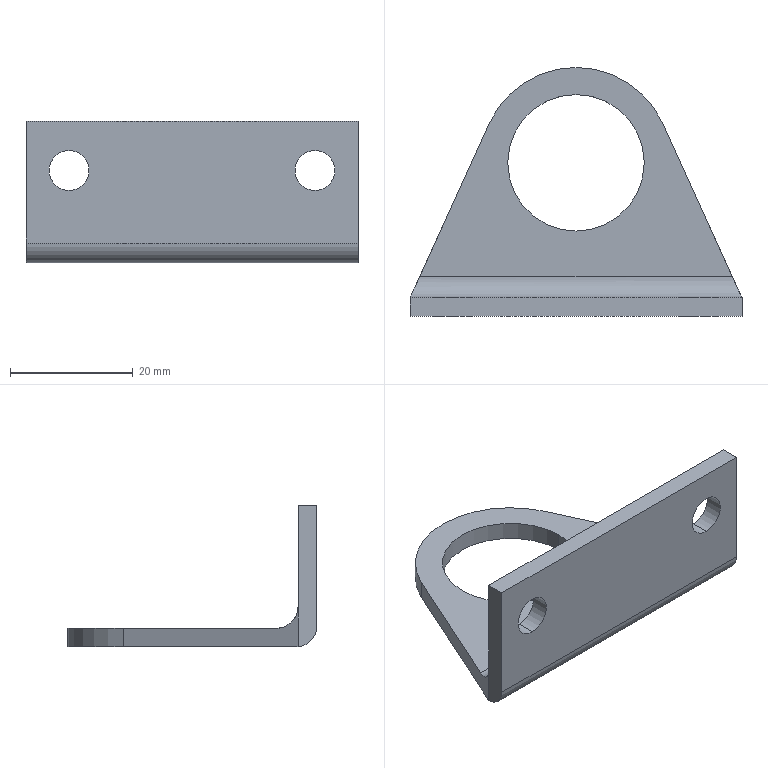Part | SolidWorks | features BaseBody 1 | 1 solid | 18 faces | box 54 x 40.5 x 23 mm | volume 6445 mm3 | cylinder 9 | plane 9 | commonest cylinder face diameters 6.5 x4 22.2 x2 6.4 x1 7 x1 31 x1
STEP:
#1=CARTESIAN_POINT('',(-11.1,0.,0.));
#2=VERTEX_POINT('',#1);
#3=CARTESIAN_POINT('',(-11.1,0.,3.));
#4=VERTEX_POINT('',#3);
#5=CARTESIAN_POINT('',(-11.1,0.,3.));
#6=DIRECTION('',(0.,0.,1.));
#7=VECTOR('',#6,1000.);
#8=LINE('',#5,#7);
#9=EDGE_CURVE('',#2,#4,#8,.T.);
#10=ORIENTED_EDGE('',*,*,#9,.F.);
#11=CARTESIAN_POINT('',(11.1,0.,0.));
#12=VERTEX_POINT('',#11);
#13=CARTESIAN_POINT('',(0.,0.,0.));
#14=DIRECTION('',(0.,0.,-1.));
#15=DIRECTION('',(1.,0.,0.));
#16=AXIS2_PLACEMENT_3D('',#13,#14,#15);
#17=CIRCLE('',#16,11.1);
#18=EDGE_CURVE('',#2,#12,#17,.T.);
#19=ORIENTED_EDGE('',*,*,#18,.T.);
#20=CARTESIAN_POINT('',(11.1,0.,3.));
#21=VERTEX_POINT('',#20);
#22=CARTESIAN_POINT('',(11.1,0.,3.));
#23=DIRECTION('',(0.,0.,1.));
#24=VECTOR('',#23,1000.);
#25=LINE('',#22,#24);
#26=EDGE_CURVE('',#12,#21,#25,.T.);
#27=ORIENTED_EDGE('',*,*,#26,.T.);
#28=CARTESIAN_POINT('',(0.,0.,3.));
#29=DIRECTION('',(0.,0.,1.));
#30=DIRECTION('',(1.,0.,0.));
#31=AXIS2_PLACEMENT_3D('',#28,#29,#30);
#32=CIRCLE('',#31,11.1);
#33=EDGE_CURVE('',#21,#4,#32,.T.);
#34=ORIENTED_EDGE('',*,*,#33,.T.);
#35=EDGE_LOOP('',(#10,#19,#27,#34));
#36=FACE_OUTER_BOUND('',#35,.T.);
#37=CARTESIAN_POINT('',(0.,0.,3.));
#38=DIRECTION('',(0.,0.,1.));
#39=DIRECTION('',(1.,0.,0.));
#40=AXIS2_PLACEMENT_3D('',#37,#38,#39);
#41=CYLINDRICAL_SURFACE('',#40,11.1);
#42=ADVANCED_FACE('',(#36),#41,.F.);
#43=CARTESIAN_POINT('',(-27.,-22.,6.5));
#44=VERTEX_POINT('',#43);
#45=CARTESIAN_POINT('',(-25.412,-18.5,3.));
#46=VERTEX_POINT('',#45);
#47=CARTESIAN_POINT('',(-27.,-22.,6.5));
#48=CARTESIAN_POINT('',(-27.,-22.,4.45));
#49=CARTESIAN_POINT('',(-26.342,-20.55,3.));
#50=CARTESIAN_POINT('',(-25.412,-18.5,3.));
#51=(BOUNDED_CURVE()B_SPLINE_CURVE(3,(#47,#48,#49,#50),.UNSPECIFIED.,.F.,.T.)B_SPLINE_CURVE_WITH_KNOTS((4,4),(3.142,4.712),.UNSPECIFIED.)CURVE()GEOMETRIC_REPRESENTATION_ITEM()RATIONAL_B_SPLINE_CURVE((1.,0.8047,0.8047,1.))REPRESENTATION_ITEM(''));
#52=EDGE_CURVE('',#44,#46,#51,.T.);
#53=ORIENTED_EDGE('',*,*,#52,.F.);
#54=CARTESIAN_POINT('',(27.,-22.,6.5));
#55=VERTEX_POINT('',#54);
#56=CARTESIAN_POINT('',(27.,-22.,6.5));
#57=DIRECTION('',(1.,0.,0.));
#58=VECTOR('',#57,1000.);
#59=LINE('',#56,#58);
#60=EDGE_CURVE('',#44,#55,#59,.T.);
#61=ORIENTED_EDGE('',*,*,#60,.T.);
#62=CARTESIAN_POINT('',(25.412,-18.5,3.));
#63=VERTEX_POINT('',#62);
#64=CARTESIAN_POINT('',(25.412,-18.5,3.));
#65=CARTESIAN_POINT('',(26.342,-20.55,3.));
#66=CARTESIAN_POINT('',(27.,-22.,4.45));
#67=CARTESIAN_POINT('',(27.,-22.,6.5));
#68=(BOUNDED_CURVE()B_SPLINE_CURVE(3,(#64,#65,#66,#67),.UNSPECIFIED.,.F.,.F.)B_SPLINE_CURVE_WITH_KNOTS((4,4),(4.712,6.283),.UNSPECIFIED.)CURVE()GEOMETRIC_REPRESENTATION_ITEM()RATIONAL_B_SPLINE_CURVE((1.,0.8047,0.8047,1.))REPRESENTATION_ITEM(''));
#69=EDGE_CURVE('',#63,#55,#68,.T.);
#70=ORIENTED_EDGE('',*,*,#69,.F.);
#71=CARTESIAN_POINT('',(27.,-18.5,3.));
#72=DIRECTION('',(-1.,0.,0.));
#73=VECTOR('',#72,1000.);
#74=LINE('',#71,#73);
#75=EDGE_CURVE('',#63,#46,#74,.T.);
#76=ORIENTED_EDGE('',*,*,#75,.T.);
#77=EDGE_LOOP('',(#53,#61,#70,#76));
#78=FACE_OUTER_BOUND('',#77,.T.);
#79=CARTESIAN_POINT('',(27.,-18.5,6.5));
#80=DIRECTION('',(1.,0.,0.));
#81=DIRECTION('',(0.,0.,-1.));
#82=AXIS2_PLACEMENT_3D('',#79,#80,#81);
#83=CYLINDRICAL_SURFACE('',#82,3.5);
#84=ADVANCED_FACE('',(#78),#83,.F.);
#85=ORIENTED_EDGE('',*,*,#33,.F.);
#86=CARTESIAN_POINT('',(0.,0.,3.));
#87=DIRECTION('',(0.,0.,1.));
#88=DIRECTION('',(1.,0.,0.));
#89=AXIS2_PLACEMENT_3D('',#86,#87,#88);
#90=CIRCLE('',#89,11.1);
#91=EDGE_CURVE('',#4,#21,#90,.T.);
#92=ORIENTED_EDGE('',*,*,#91,.F.);
#93=EDGE_LOOP('',(#85,#92));
#94=FACE_BOUND('',#93,.T.);
#95=ORIENTED_EDGE('',*,*,#75,.F.);
#96=CARTESIAN_POINT('',(14.116,6.403,3.));
#97=VERTEX_POINT('',#96);
#98=CARTESIAN_POINT('',(14.116,6.403,3.));
#99=DIRECTION('',(0.4131,-0.9107,0.));
#100=VECTOR('',#99,1000.);
#101=LINE('',#98,#100);
#102=EDGE_CURVE('',#97,#63,#101,.T.);
#103=ORIENTED_EDGE('',*,*,#102,.F.);
#104=CARTESIAN_POINT('',(-14.116,6.403,3.));
#105=VERTEX_POINT('',#104);
#106=CARTESIAN_POINT('',(0.,0.,3.));
#107=DIRECTION('',(0.,0.,-1.));
#108=DIRECTION('',(1.,0.,0.));
#109=AXIS2_PLACEMENT_3D('',#106,#107,#108);
#110=CIRCLE('',#109,15.5);
#111=EDGE_CURVE('',#105,#97,#110,.T.);
#112=ORIENTED_EDGE('',*,*,#111,.F.);
#113=CARTESIAN_POINT('',(-27.,-22.,3.));
#114=DIRECTION('',(0.4131,0.9107,0.));
#115=VECTOR('',#114,1000.);
#116=LINE('',#113,#115);
#117=EDGE_CURVE('',#46,#105,#116,.T.);
#118=ORIENTED_EDGE('',*,*,#117,.F.);
#119=EDGE_LOOP('',(#95,#103,#112,#118));
#120=FACE_OUTER_BOUND('',#119,.T.);
#121=CARTESIAN_POINT('',(27.,15.5,3.));
#122=DIRECTION('',(0.,0.,-1.));
#123=DIRECTION('',(0.,-1.,0.));
#124=AXIS2_PLACEMENT_3D('',#121,#122,#123);
#125=PLANE('',#124);
#126=ADVANCED_FACE('',(#94,#120),#125,.F.);
#127=ORIENTED_EDGE('',*,*,#111,.T.);
#128=CARTESIAN_POINT('',(14.116,6.403,0.));
#129=VERTEX_POINT('',#128);
#130=CARTESIAN_POINT('',(14.116,6.403,9.));
#131=DIRECTION('',(0.,0.,1.));
#132=VECTOR('',#131,1000.);
#133=LINE('',#130,#132);
#134=EDGE_CURVE('',#129,#97,#133,.T.);
#135=ORIENTED_EDGE('',*,*,#134,.F.);
#136=CARTESIAN_POINT('',(-14.116,6.403,0.));
#137=VERTEX_POINT('',#136);
#138=CARTESIAN_POINT('',(0.,0.,0.));
#139=DIRECTION('',(0.,0.,1.));
#140=DIRECTION('',(1.,0.,0.));
#141=AXIS2_PLACEMENT_3D('',#138,#139,#140);
#142=CIRCLE('',#141,15.5);
#143=EDGE_CURVE('',#129,#137,#142,.T.);
#144=ORIENTED_EDGE('',*,*,#143,.T.);
#145=CARTESIAN_POINT('',(-14.116,6.403,9.));
#146=DIRECTION('',(0.,0.,-1.));
#147=VECTOR('',#146,1000.);
#148=LINE('',#145,#147);
#149=EDGE_CURVE('',#105,#137,#148,.T.);
#150=ORIENTED_EDGE('',*,*,#149,.F.);
#151=EDGE_LOOP('',(#127,#135,#144,#150));
#152=FACE_OUTER_BOUND('',#151,.T.);
#153=CARTESIAN_POINT('',(0.,0.,9.));
#154=DIRECTION('',(0.,0.,1.));
#155=DIRECTION('',(1.,0.,0.));
#156=AXIS2_PLACEMENT_3D('',#153,#154,#155);
#157=CYLINDRICAL_SURFACE('',#156,15.5);
#158=ADVANCED_FACE('',(#152),#157,.T.);
#159=ORIENTED_EDGE('',*,*,#69,.T.);
#160=CARTESIAN_POINT('',(27.,-22.,0.006256));
#161=VERTEX_POINT('',#160);
#162=CARTESIAN_POINT('',(27.,-22.,3.2));
#163=DIRECTION('',(0.,0.,1.));
#164=VECTOR('',#163,1000.);
#165=LINE('',#162,#164);
#166=EDGE_CURVE('',#161,#55,#165,.T.);
#167=ORIENTED_EDGE('',*,*,#166,.F.);
#168=CARTESIAN_POINT('',(26.909,-21.8,0.));
#169=VERTEX_POINT('',#168);
#170=CARTESIAN_POINT('',(27.,-22.,0.006256));
#171=CARTESIAN_POINT('',(26.97,-21.933,0.002086));
#172=CARTESIAN_POINT('',(26.94,-21.867,0.));
#173=CARTESIAN_POINT('',(26.909,-21.8,0.));
#174=(BOUNDED_CURVE()B_SPLINE_CURVE(3,(#170,#171,#172,#173),.UNSPECIFIED.,.F.,.F.)B_SPLINE_CURVE_WITH_KNOTS((4,4),(1.508,1.571),.UNSPECIFIED.)CURVE()GEOMETRIC_REPRESENTATION_ITEM()RATIONAL_B_SPLINE_CURVE((1.,0.9997,0.9997,1.))REPRESENTATION_ITEM(''));
#175=EDGE_CURVE('',#161,#169,#174,.T.);
#176=ORIENTED_EDGE('',*,*,#175,.T.);
#177=CARTESIAN_POINT('',(26.909,-21.8,0.));
#178=DIRECTION('',(-0.4131,0.9107,0.));
#179=VECTOR('',#178,1000.);
#180=LINE('',#177,#179);
#181=EDGE_CURVE('',#169,#129,#180,.T.);
#182=ORIENTED_EDGE('',*,*,#181,.T.);
#183=ORIENTED_EDGE('',*,*,#134,.T.);
#184=ORIENTED_EDGE('',*,*,#102,.T.);
#185=EDGE_LOOP('',(#159,#167,#176,#182,#183,#184));
#186=FACE_OUTER_BOUND('',#185,.T.);
#187=CARTESIAN_POINT('',(14.116,6.403,9.));
#188=DIRECTION('',(0.9107,0.4131,0.));
#189=DIRECTION('',(0.,0.,-1.));
#190=AXIS2_PLACEMENT_3D('',#187,#188,#189);
#191=PLANE('',#190);
#192=ADVANCED_FACE('',(#186),#191,.T.);
#193=CARTESIAN_POINT('',(0.,0.,0.));
#194=DIRECTION('',(0.,0.,-1.));
#195=DIRECTION('',(1.,0.,0.));
#196=AXIS2_PLACEMENT_3D('',#193,#194,#195);
#197=CIRCLE('',#196,11.1);
#198=EDGE_CURVE('',#12,#2,#197,.T.);
#199=ORIENTED_EDGE('',*,*,#198,.F.);
#200=ORIENTED_EDGE('',*,*,#18,.F.);
#201=EDGE_LOOP('',(#199,#200));
#202=FACE_BOUND('',#201,.T.);
#203=ORIENTED_EDGE('',*,*,#143,.F.);
#204=ORIENTED_EDGE('',*,*,#181,.F.);
#205=CARTESIAN_POINT('',(-26.909,-21.8,0.));
#206=VERTEX_POINT('',#205);
#207=CARTESIAN_POINT('',(27.,-21.8,0.));
#208=DIRECTION('',(1.,0.,0.));
#209=VECTOR('',#208,1000.);
#210=LINE('',#207,#209);
#211=EDGE_CURVE('',#206,#169,#210,.T.);
#212=ORIENTED_EDGE('',*,*,#211,.F.);
#213=CARTESIAN_POINT('',(-27.,-22.,0.));
#214=DIRECTION('',(-0.4131,-0.9107,0.));
#215=VECTOR('',#214,1000.);
#216=LINE('',#213,#215);
#217=EDGE_CURVE('',#137,#206,#216,.T.);
#218=ORIENTED_EDGE('',*,*,#217,.F.);
#219=EDGE_LOOP('',(#203,#204,#212,#218));
#220=FACE_OUTER_BOUND('',#219,.T.);
#221=CARTESIAN_POINT('',(27.,-21.8,0.));
#222=DIRECTION('',(0.,0.,1.));
#223=DIRECTION('',(1.,0.,0.));
#224=AXIS2_PLACEMENT_3D('',#221,#222,#223);
#225=PLANE('',#224);
#226=ADVANCED_FACE('',(#202,#220),#225,.F.);
#227=CARTESIAN_POINT('',(-20.,-22.,18.25));
#228=VERTEX_POINT('',#227);
#229=CARTESIAN_POINT('',(-20.,-22.,11.75));
#230=VERTEX_POINT('',#229);
#231=CARTESIAN_POINT('',(-20.,-22.,15.));
#232=DIRECTION('',(0.,-1.,0.));
#233=DIRECTION('',(0.,0.,1.));
#234=AXIS2_PLACEMENT_3D('',#231,#232,#233);
#235=CIRCLE('',#234,3.25);
#236=EDGE_CURVE('',#228,#230,#235,.T.);
#237=ORIENTED_EDGE('',*,*,#236,.T.);
#238=CARTESIAN_POINT('',(-20.,-22.,15.));
#239=DIRECTION('',(0.,-1.,0.));
#240=DIRECTION('',(0.,0.,1.));
#241=AXIS2_PLACEMENT_3D('',#238,#239,#240);
#242=CIRCLE('',#241,3.25);
#243=EDGE_CURVE('',#230,#228,#242,.T.);
#244=ORIENTED_EDGE('',*,*,#243,.T.);
#245=EDGE_LOOP('',(#237,#244));
#246=FACE_BOUND('',#245,.T.);
#247=CARTESIAN_POINT('',(20.,-22.,18.25));
#248=VERTEX_POINT('',#247);
#249=CARTESIAN_POINT('',(20.,-22.,11.75));
#250=VERTEX_POINT('',#249);
#251=CARTESIAN_POINT('',(20.,-22.,15.));
#252=DIRECTION('',(0.,-1.,0.));
#253=DIRECTION('',(0.,0.,1.));
#254=AXIS2_PLACEMENT_3D('',#251,#252,#253);
#255=CIRCLE('',#254,3.25);
#256=EDGE_CURVE('',#248,#250,#255,.T.);
#257=ORIENTED_EDGE('',*,*,#256,.T.);
#258=CARTESIAN_POINT('',(20.,-22.,15.));
#259=DIRECTION('',(0.,-1.,0.));
#260=DIRECTION('',(0.,0.,1.));
#261=AXIS2_PLACEMENT_3D('',#258,#259,#260);
#262=CIRCLE('',#261,3.25);
#263=EDGE_CURVE('',#250,#248,#262,.T.);
#264=ORIENTED_EDGE('',*,*,#263,.T.);
#265=EDGE_LOOP('',(#257,#264));
#266=FACE_BOUND('',#265,.T.);
#267=CARTESIAN_POINT('',(-27.,-22.,23.));
#268=VERTEX_POINT('',#267);
#269=CARTESIAN_POINT('',(27.,-22.,23.));
#270=VERTEX_POINT('',#269);
#271=CARTESIAN_POINT('',(27.,-22.,23.));
#272=DIRECTION('',(1.,0.,0.));
#273=VECTOR('',#272,1000.);
#274=LINE('',#271,#273);
#275=EDGE_CURVE('',#268,#270,#274,.T.);
#276=ORIENTED_EDGE('',*,*,#275,.T.);
#277=CARTESIAN_POINT('',(27.,-22.,3.2));
#278=DIRECTION('',(0.,0.,1.));
#279=VECTOR('',#278,1000.);
#280=LINE('',#277,#279);
#281=EDGE_CURVE('',#55,#270,#280,.T.);
#282=ORIENTED_EDGE('',*,*,#281,.F.);
#283=ORIENTED_EDGE('',*,*,#60,.F.);
#284=CARTESIAN_POINT('',(-27.,-22.,3.2));
#285=DIRECTION('',(0.,0.,1.));
#286=VECTOR('',#285,1000.);
#287=LINE('',#284,#286);
#288=EDGE_CURVE('',#44,#268,#287,.T.);
#289=ORIENTED_EDGE('',*,*,#288,.T.);
#290=EDGE_LOOP('',(#276,#282,#283,#289));
#291=FACE_OUTER_BOUND('',#290,.T.);
#292=CARTESIAN_POINT('',(27.,-22.,6.5));
#293=DIRECTION('',(0.,-1.,0.));
#294=DIRECTION('',(0.,0.,-1.));
#295=AXIS2_PLACEMENT_3D('',#292,#293,#294);
#296=PLANE('',#295);
#297=ADVANCED_FACE('',(#246,#266,#291),#296,.F.);
#298=ORIENTED_EDGE('',*,*,#149,.T.);
#299=ORIENTED_EDGE('',*,*,#217,.T.);
#300=CARTESIAN_POINT('',(-27.,-22.,0.006256));
#301=VERTEX_POINT('',#300);
#302=CARTESIAN_POINT('',(-27.,-22.,0.006256));
#303=CARTESIAN_POINT('',(-26.97,-21.933,0.002086));
#304=CARTESIAN_POINT('',(-26.94,-21.867,0.));
#305=CARTESIAN_POINT('',(-26.909,-21.8,0.));
#306=(BOUNDED_CURVE()B_SPLINE_CURVE(3,(#302,#303,#304,#305),.UNSPECIFIED.,.F.,.F.)B_SPLINE_CURVE_WITH_KNOTS((4,4),(4.65,4.712),.UNSPECIFIED.)CURVE()GEOMETRIC_REPRESENTATION_ITEM()RATIONAL_B_SPLINE_CURVE((1.,0.9997,0.9997,1.))REPRESENTATION_ITEM(''));
#307=EDGE_CURVE('',#301,#206,#306,.T.);
#308=ORIENTED_EDGE('',*,*,#307,.F.);
#309=CARTESIAN_POINT('',(-27.,-22.,3.2));
#310=DIRECTION('',(0.,0.,1.));
#311=VECTOR('',#310,1000.);
#312=LINE('',#309,#311);
#313=EDGE_CURVE('',#301,#44,#312,.T.);
#314=ORIENTED_EDGE('',*,*,#313,.T.);
#315=ORIENTED_EDGE('',*,*,#52,.T.);
#316=ORIENTED_EDGE('',*,*,#117,.T.);
#317=EDGE_LOOP('',(#298,#299,#308,#314,#315,#316));
#318=FACE_OUTER_BOUND('',#317,.T.);
#319=CARTESIAN_POINT('',(-27.,-22.,9.));
#320=DIRECTION('',(-0.9107,0.4131,0.));
#321=DIRECTION('',(0.,0.,1.));
#322=AXIS2_PLACEMENT_3D('',#319,#320,#321);
#323=PLANE('',#322);
#324=ADVANCED_FACE('',(#318),#323,.T.);
#325=CARTESIAN_POINT('',(-20.,-25.,11.75));
#326=VERTEX_POINT('',#325);
#327=CARTESIAN_POINT('',(-20.,-25.,11.75));
#328=DIRECTION('',(0.,1.,0.));
#329=VECTOR('',#328,1000.);
#330=LINE('',#327,#329);
#331=EDGE_CURVE('',#326,#230,#330,.T.);
#332=ORIENTED_EDGE('',*,*,#331,.F.);
#333=CARTESIAN_POINT('',(-20.,-25.,18.25));
#334=VERTEX_POINT('',#333);
#335=CARTESIAN_POINT('',(-20.,-25.,15.));
#336=DIRECTION('',(0.,-1.,0.));
#337=DIRECTION('',(0.,0.,1.));
#338=AXIS2_PLACEMENT_3D('',#335,#336,#337);
#339=CIRCLE('',#338,3.25);
#340=EDGE_CURVE('',#326,#334,#339,.T.);
#341=ORIENTED_EDGE('',*,*,#340,.T.);
#342=CARTESIAN_POINT('',(-20.,-25.,18.25));
#343=DIRECTION('',(0.,1.,0.));
#344=VECTOR('',#343,1000.);
#345=LINE('',#342,#344);
#346=EDGE_CURVE('',#334,#228,#345,.T.);
#347=ORIENTED_EDGE('',*,*,#346,.T.);
#348=ORIENTED_EDGE('',*,*,#243,.F.);
#349=EDGE_LOOP('',(#332,#341,#347,#348));
#350=FACE_OUTER_BOUND('',#349,.T.);
#351=CARTESIAN_POINT('',(-20.,-25.,15.));
#352=DIRECTION('',(0.,1.,0.));
#353=DIRECTION('',(0.,0.,1.));
#354=AXIS2_PLACEMENT_3D('',#351,#352,#353);
#355=CYLINDRICAL_SURFACE('',#354,3.25);
#356=ADVANCED_FACE('',(#350),#355,.F.);
#357=CARTESIAN_POINT('',(20.,-25.,11.75));
#358=VERTEX_POINT('',#357);
#359=CARTESIAN_POINT('',(20.,-25.,11.75));
#360=DIRECTION('',(0.,1.,0.));
#361=VECTOR('',#360,1000.);
#362=LINE('',#359,#361);
#363=EDGE_CURVE('',#358,#250,#362,.T.);
#364=ORIENTED_EDGE('',*,*,#363,.F.);
#365=CARTESIAN_POINT('',(20.,-25.,18.25));
#366=VERTEX_POINT('',#365);
#367=CARTESIAN_POINT('',(20.,-25.,15.));
#368=DIRECTION('',(0.,-1.,0.));
#369=DIRECTION('',(0.,0.,1.));
#370=AXIS2_PLACEMENT_3D('',#367,#368,#369);
#371=CIRCLE('',#370,3.25);
#372=EDGE_CURVE('',#358,#366,#371,.T.);
#373=ORIENTED_EDGE('',*,*,#372,.T.);
#374=CARTESIAN_POINT('',(20.,-25.,18.25));
#375=DIRECTION('',(0.,1.,0.));
#376=VECTOR('',#375,1000.);
#377=LINE('',#374,#376);
#378=EDGE_CURVE('',#366,#248,#377,.T.);
#379=ORIENTED_EDGE('',*,*,#378,.T.);
#380=ORIENTED_EDGE('',*,*,#263,.F.);
#381=EDGE_LOOP('',(#364,#373,#379,#380));
#382=FACE_OUTER_BOUND('',#381,.T.);
#383=CARTESIAN_POINT('',(20.,-25.,15.));
#384=DIRECTION('',(0.,1.,0.));
#385=DIRECTION('',(0.,0.,1.));
#386=AXIS2_PLACEMENT_3D('',#383,#384,#385);
#387=CYLINDRICAL_SURFACE('',#386,3.25);
#388=ADVANCED_FACE('',(#382),#387,.F.);
#389=CARTESIAN_POINT('',(-27.,-25.,23.));
#390=VERTEX_POINT('',#389);
#391=CARTESIAN_POINT('',(27.,-25.,23.));
#392=VERTEX_POINT('',#391);
#393=CARTESIAN_POINT('',(27.,-25.,23.));
#394=DIRECTION('',(1.,0.,0.));
#395=VECTOR('',#394,1000.);
#396=LINE('',#393,#395);
#397=EDGE_CURVE('',#390,#392,#396,.T.);
#398=ORIENTED_EDGE('',*,*,#397,.T.);
#399=CARTESIAN_POINT('',(27.,-21.8,23.));
#400=DIRECTION('',(0.,-1.,0.));
#401=VECTOR('',#400,1000.);
#402=LINE('',#399,#401);
#403=EDGE_CURVE('',#270,#392,#402,.T.);
#404=ORIENTED_EDGE('',*,*,#403,.F.);
#405=ORIENTED_EDGE('',*,*,#275,.F.);
#406=CARTESIAN_POINT('',(-27.,-21.8,23.));
#407=DIRECTION('',(0.,-1.,0.));
#408=VECTOR('',#407,1000.);
#409=LINE('',#406,#408);
#410=EDGE_CURVE('',#268,#390,#409,.T.);
#411=ORIENTED_EDGE('',*,*,#410,.T.);
#412=EDGE_LOOP('',(#398,#404,#405,#411));
#413=FACE_OUTER_BOUND('',#412,.T.);
#414=CARTESIAN_POINT('',(27.,-22.,23.));
#415=DIRECTION('',(0.,0.,-1.));
#416=DIRECTION('',(0.,-1.,0.));
#417=AXIS2_PLACEMENT_3D('',#414,#415,#416);
#418=PLANE('',#417);
#419=ADVANCED_FACE('',(#413),#418,.F.);
#420=ORIENTED_EDGE('',*,*,#403,.T.);
#421=CARTESIAN_POINT('',(27.,-25.,3.2));
#422=VERTEX_POINT('',#421);
#423=CARTESIAN_POINT('',(27.,-25.,23.));
#424=DIRECTION('',(0.,0.,-1.));
#425=VECTOR('',#424,1000.);
#426=LINE('',#423,#425);
#427=EDGE_CURVE('',#392,#422,#426,.T.);
#428=ORIENTED_EDGE('',*,*,#427,.T.);
#429=CARTESIAN_POINT('',(27.,-21.8,3.2));
#430=DIRECTION('',(-1.,0.,0.));
#431=DIRECTION('',(0.,0.,-1.));
#432=AXIS2_PLACEMENT_3D('',#429,#430,#431);
#433=CIRCLE('',#432,3.2);
#434=EDGE_CURVE('',#161,#422,#433,.T.);
#435=ORIENTED_EDGE('',*,*,#434,.F.);
#436=ORIENTED_EDGE('',*,*,#166,.T.);
#437=ORIENTED_EDGE('',*,*,#281,.T.);
#438=EDGE_LOOP('',(#420,#428,#435,#436,#437));
#439=FACE_OUTER_BOUND('',#438,.T.);
#440=CARTESIAN_POINT('',(27.,-21.8,3.2));
#441=DIRECTION('',(1.,0.,0.));
#442=DIRECTION('',(0.,1.,0.));
#443=AXIS2_PLACEMENT_3D('',#440,#441,#442);
#444=PLANE('',#443);
#445=ADVANCED_FACE('',(#439),#444,.T.);
#446=CARTESIAN_POINT('',(-27.,-25.,3.2));
#447=VERTEX_POINT('',#446);
#448=CARTESIAN_POINT('',(27.,-25.,3.2));
#449=DIRECTION('',(-1.,0.,0.));
#450=VECTOR('',#449,1000.);
#451=LINE('',#448,#450);
#452=EDGE_CURVE('',#422,#447,#451,.T.);
#453=ORIENTED_EDGE('',*,*,#452,.T.);
#454=CARTESIAN_POINT('',(-27.,-21.8,3.2));
#455=DIRECTION('',(1.,0.,0.));
#456=DIRECTION('',(0.,0.,-1.));
#457=AXIS2_PLACEMENT_3D('',#454,#455,#456);
#458=CIRCLE('',#457,3.2);
#459=EDGE_CURVE('',#447,#301,#458,.T.);
#460=ORIENTED_EDGE('',*,*,#459,.T.);
#461=ORIENTED_EDGE('',*,*,#307,.T.);
#462=ORIENTED_EDGE('',*,*,#211,.T.);
#463=ORIENTED_EDGE('',*,*,#175,.F.);
#464=ORIENTED_EDGE('',*,*,#434,.T.);
#465=EDGE_LOOP('',(#453,#460,#461,#462,#463,#464));
#466=FACE_OUTER_BOUND('',#465,.T.);
#467=CARTESIAN_POINT('',(27.,-21.8,3.2));
#468=DIRECTION('',(1.,0.,0.));
#469=DIRECTION('',(0.,0.,-1.));
#470=AXIS2_PLACEMENT_3D('',#467,#468,#469);
#471=CYLINDRICAL_SURFACE('',#470,3.2);
#472=ADVANCED_FACE('',(#466),#471,.T.);
#473=ORIENTED_EDGE('',*,*,#459,.F.);
#474=CARTESIAN_POINT('',(-27.,-25.,23.));
#475=DIRECTION('',(0.,0.,1.));
#476=VECTOR('',#475,1000.);
#477=LINE('',#474,#476);
#478=EDGE_CURVE('',#447,#390,#477,.T.);
#479=ORIENTED_EDGE('',*,*,#478,.T.);
#480=ORIENTED_EDGE('',*,*,#410,.F.);
#481=ORIENTED_EDGE('',*,*,#288,.F.);
#482=ORIENTED_EDGE('',*,*,#313,.F.);
#483=EDGE_LOOP('',(#473,#479,#480,#481,#482));
#484=FACE_OUTER_BOUND('',#483,.T.);
#485=CARTESIAN_POINT('',(-27.,-21.8,3.2));
#486=DIRECTION('',(1.,0.,0.));
#487=DIRECTION('',(0.,1.,0.));
#488=AXIS2_PLACEMENT_3D('',#485,#486,#487);
#489=PLANE('',#488);
#490=ADVANCED_FACE('',(#484),#489,.F.);
#491=CARTESIAN_POINT('',(-20.,-25.,15.));
#492=DIRECTION('',(0.,-1.,0.));
#493=DIRECTION('',(0.,0.,1.));
#494=AXIS2_PLACEMENT_3D('',#491,#492,#493);
#495=CIRCLE('',#494,3.25);
#496=EDGE_CURVE('',#334,#326,#495,.T.);
#497=ORIENTED_EDGE('',*,*,#496,.F.);
#498=ORIENTED_EDGE('',*,*,#340,.F.);
#499=EDGE_LOOP('',(#497,#498));
#500=FACE_BOUND('',#499,.T.);
#501=CARTESIAN_POINT('',(20.,-25.,15.));
#502=DIRECTION('',(0.,-1.,0.));
#503=DIRECTION('',(0.,0.,1.));
#504=AXIS2_PLACEMENT_3D('',#501,#502,#503);
#505=CIRCLE('',#504,3.25);
#506=EDGE_CURVE('',#366,#358,#505,.T.);
#507=ORIENTED_EDGE('',*,*,#506,.F.);
#508=ORIENTED_EDGE('',*,*,#372,.F.);
#509=EDGE_LOOP('',(#507,#508));
#510=FACE_BOUND('',#509,.T.);
#511=ORIENTED_EDGE('',*,*,#452,.F.);
#512=ORIENTED_EDGE('',*,*,#427,.F.);
#513=ORIENTED_EDGE('',*,*,#397,.F.);
#514=ORIENTED_EDGE('',*,*,#478,.F.);
#515=EDGE_LOOP('',(#511,#512,#513,#514));
#516=FACE_OUTER_BOUND('',#515,.T.);
#517=CARTESIAN_POINT('',(27.,-25.,23.));
#518=DIRECTION('',(0.,1.,0.));
#519=DIRECTION('',(1.,0.,0.));
#520=AXIS2_PLACEMENT_3D('',#517,#518,#519);
#521=PLANE('',#520);
#522=ADVANCED_FACE('',(#500,#510,#516),#521,.F.);
#523=ORIENTED_EDGE('',*,*,#198,.T.);
#524=ORIENTED_EDGE('',*,*,#9,.T.);
#525=ORIENTED_EDGE('',*,*,#91,.T.);
#526=ORIENTED_EDGE('',*,*,#26,.F.);
#527=EDGE_LOOP('',(#523,#524,#525,#526));
#528=FACE_OUTER_BOUND('',#527,.T.);
#529=CARTESIAN_POINT('',(0.,0.,3.));
#530=DIRECTION('',(0.,0.,1.));
#531=DIRECTION('',(1.,0.,0.));
#532=AXIS2_PLACEMENT_3D('',#529,#530,#531);
#533=CYLINDRICAL_SURFACE('',#532,11.1);
#534=ADVANCED_FACE('',(#528),#533,.F.);
#535=ORIENTED_EDGE('',*,*,#496,.T.);
#536=ORIENTED_EDGE('',*,*,#331,.T.);
#537=ORIENTED_EDGE('',*,*,#236,.F.);
#538=ORIENTED_EDGE('',*,*,#346,.F.);
#539=EDGE_LOOP('',(#535,#536,#537,#538));
#540=FACE_OUTER_BOUND('',#539,.T.);
#541=CARTESIAN_POINT('',(-20.,-25.,15.));
#542=DIRECTION('',(0.,1.,0.));
#543=DIRECTION('',(0.,0.,1.));
#544=AXIS2_PLACEMENT_3D('',#541,#542,#543);
#545=CYLINDRICAL_SURFACE('',#544,3.25);
#546=ADVANCED_FACE('',(#540),#545,.F.);
#547=ORIENTED_EDGE('',*,*,#506,.T.);
#548=ORIENTED_EDGE('',*,*,#363,.T.);
#549=ORIENTED_EDGE('',*,*,#256,.F.);
#550=ORIENTED_EDGE('',*,*,#378,.F.);
#551=EDGE_LOOP('',(#547,#548,#549,#550));
#552=FACE_OUTER_BOUND('',#551,.T.);
#553=CARTESIAN_POINT('',(20.,-25.,15.));
#554=DIRECTION('',(0.,1.,0.));
#555=DIRECTION('',(0.,0.,1.));
#556=AXIS2_PLACEMENT_3D('',#553,#554,#555);
#557=CYLINDRICAL_SURFACE('',#556,3.25);
#558=ADVANCED_FACE('',(#552),#557,.F.);
#559=CLOSED_SHELL('',(#42,#84,#126,#158,#192,#226,#297,#324,#356,#388,#419,#445,#472,#490,#522,#534,#546,#558));
#560=MANIFOLD_SOLID_BREP('',#559);
#561=CARTESIAN_POINT('',(0.,0.,0.));
#562=DIRECTION('',(0.,0.,1.));
#563=DIRECTION('',(1.,0.,0.));
#564=AXIS2_PLACEMENT_3D('',#561,#562,#563);
#565=(LENGTH_UNIT()NAMED_UNIT(*)SI_UNIT(.MILLI.,.METRE.));
#566=UNCERTAINTY_MEASURE_WITH_UNIT(LENGTH_MEASURE(0.00001),#565,'','');
#567=(NAMED_UNIT(*)PLANE_ANGLE_UNIT()SI_UNIT($,.RADIAN.));
#568=(NAMED_UNIT(*)SI_UNIT($,.STERADIAN.)SOLID_ANGLE_UNIT());
#569=(GEOMETRIC_REPRESENTATION_CONTEXT(3)GLOBAL_UNCERTAINTY_ASSIGNED_CONTEXT((#566))GLOBAL_UNIT_ASSIGNED_CONTEXT((#565,#567,#568))REPRESENTATION_CONTEXT('',''));
#570=ADVANCED_BREP_SHAPE_REPRESENTATION('',(#560,#564),#569);